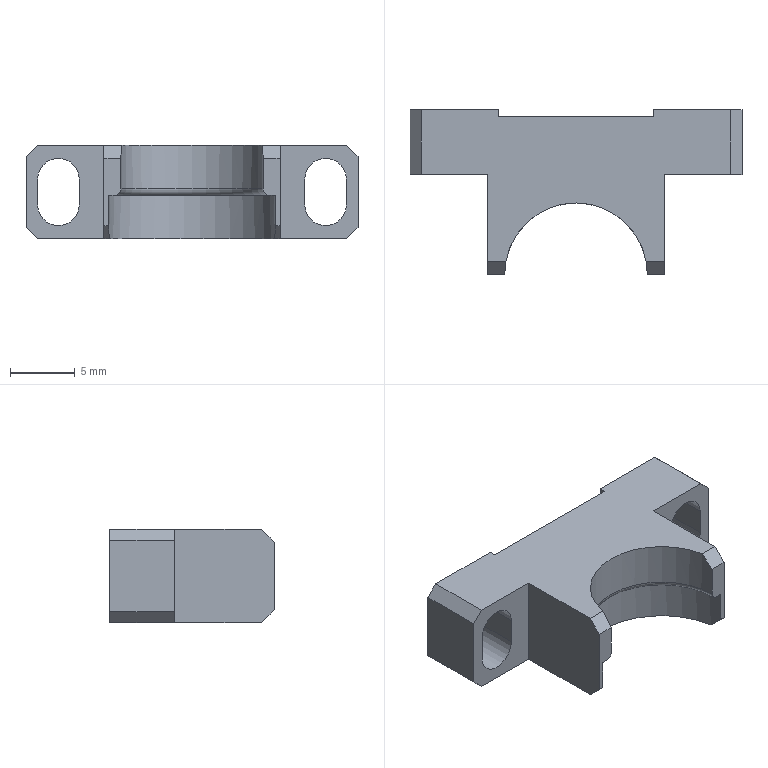Part | SolidWorks | features ICE 7, Chamfer 2, MoveFace 2, Extrusion 1, Fillet 1 | 1 solid | 35 faces | box 25.6 x 12.7 x 7.2 mm | volume 1076 mm3 | plane 28 | cylinder 6 | torus 1 | commonest cylinder face diameters 3.2 x4 11 x1 12.9 x1
STEP:
#1=CARTESIAN_POINT('',(12.8,12.7,5.995));
#2=VERTEX_POINT('',#1);
#3=CARTESIAN_POINT('',(12.8,12.7,0.505));
#4=VERTEX_POINT('',#3);
#5=CARTESIAN_POINT('',(12.8,12.7,0.));
#6=DIRECTION('',(0.,0.,-1.));
#7=VECTOR('',#6,1000.);
#8=LINE('',#5,#7);
#9=EDGE_CURVE('',#2,#4,#8,.T.);
#10=ORIENTED_EDGE('',*,*,#9,.T.);
#11=CARTESIAN_POINT('',(11.945,12.7,-0.35));
#12=VERTEX_POINT('',#11);
#13=CARTESIAN_POINT('',(9.547,12.7,-2.747));
#14=DIRECTION('',(-0.7071,0.,-0.7071));
#15=VECTOR('',#14,1000.);
#16=LINE('',#13,#15);
#17=EDGE_CURVE('',#4,#12,#16,.T.);
#18=ORIENTED_EDGE('',*,*,#17,.T.);
#19=CARTESIAN_POINT('',(6.,12.7,-0.35));
#20=VERTEX_POINT('',#19);
#21=CARTESIAN_POINT('',(0.,12.7,-0.35));
#22=DIRECTION('',(-1.,0.,0.));
#23=VECTOR('',#22,1000.);
#24=LINE('',#21,#23);
#25=EDGE_CURVE('',#12,#20,#24,.T.);
#26=ORIENTED_EDGE('',*,*,#25,.T.);
#27=CARTESIAN_POINT('',(6.,12.7,6.85));
#28=VERTEX_POINT('',#27);
#29=CARTESIAN_POINT('',(6.,12.7,0.));
#30=DIRECTION('',(0.,0.,-1.));
#31=VECTOR('',#30,1000.);
#32=LINE('',#29,#31);
#33=EDGE_CURVE('',#28,#20,#32,.T.);
#34=ORIENTED_EDGE('',*,*,#33,.F.);
#35=CARTESIAN_POINT('',(11.945,12.7,6.85));
#36=VERTEX_POINT('',#35);
#37=CARTESIAN_POINT('',(0.,12.7,6.85));
#38=DIRECTION('',(-1.,0.,0.));
#39=VECTOR('',#38,1000.);
#40=LINE('',#37,#39);
#41=EDGE_CURVE('',#36,#28,#40,.T.);
#42=ORIENTED_EDGE('',*,*,#41,.F.);
#43=CARTESIAN_POINT('',(12.797,12.7,5.997));
#44=DIRECTION('',(0.7071,0.,-0.7071));
#45=VECTOR('',#44,1000.);
#46=LINE('',#43,#45);
#47=EDGE_CURVE('',#36,#2,#46,.T.);
#48=ORIENTED_EDGE('',*,*,#47,.T.);
#49=EDGE_LOOP('',(#10,#18,#26,#34,#42,#48));
#50=FACE_OUTER_BOUND('',#49,.T.);
#51=CARTESIAN_POINT('',(8.7,12.7,2.25));
#52=VERTEX_POINT('',#51);
#53=CARTESIAN_POINT('',(11.9,12.7,2.25));
#54=VERTEX_POINT('',#53);
#55=CARTESIAN_POINT('',(10.3,12.7,2.25));
#56=DIRECTION('',(0.,-1.,0.));
#57=DIRECTION('',(1.,0.,0.));
#58=AXIS2_PLACEMENT_3D('',#55,#56,#57);
#59=CIRCLE('',#58,1.6);
#60=EDGE_CURVE('',#52,#54,#59,.T.);
#61=ORIENTED_EDGE('',*,*,#60,.T.);
#62=CARTESIAN_POINT('',(11.9,12.7,4.25));
#63=VERTEX_POINT('',#62);
#64=CARTESIAN_POINT('',(11.9,12.7,2.25));
#65=DIRECTION('',(0.,0.,1.));
#66=VECTOR('',#65,1000.);
#67=LINE('',#64,#66);
#68=EDGE_CURVE('',#54,#63,#67,.T.);
#69=ORIENTED_EDGE('',*,*,#68,.T.);
#70=CARTESIAN_POINT('',(8.7,12.7,4.25));
#71=VERTEX_POINT('',#70);
#72=CARTESIAN_POINT('',(10.3,12.7,4.25));
#73=DIRECTION('',(0.,-1.,0.));
#74=DIRECTION('',(1.,0.,0.));
#75=AXIS2_PLACEMENT_3D('',#72,#73,#74);
#76=CIRCLE('',#75,1.6);
#77=EDGE_CURVE('',#63,#71,#76,.T.);
#78=ORIENTED_EDGE('',*,*,#77,.T.);
#79=CARTESIAN_POINT('',(8.7,12.7,2.25));
#80=DIRECTION('',(0.,0.,-1.));
#81=VECTOR('',#80,1000.);
#82=LINE('',#79,#81);
#83=EDGE_CURVE('',#71,#52,#82,.T.);
#84=ORIENTED_EDGE('',*,*,#83,.T.);
#85=EDGE_LOOP('',(#61,#69,#78,#84));
#86=FACE_BOUND('',#85,.T.);
#87=CARTESIAN_POINT('',(6.8,12.7,0.));
#88=DIRECTION('',(0.,1.,0.));
#89=DIRECTION('',(-1.,0.,0.));
#90=AXIS2_PLACEMENT_3D('',#87,#88,#89);
#91=PLANE('',#90);
#92=ADVANCED_FACE('',(#50,#86),#91,.T.);
#93=CARTESIAN_POINT('',(-6.8,0.,0.65));
#94=VERTEX_POINT('',#93);
#95=CARTESIAN_POINT('',(-6.8,0.,5.85));
#96=VERTEX_POINT('',#95);
#97=CARTESIAN_POINT('',(-6.8,0.,0.));
#98=DIRECTION('',(0.,0.,1.));
#99=VECTOR('',#98,1000.);
#100=LINE('',#97,#99);
#101=EDGE_CURVE('',#94,#96,#100,.T.);
#102=ORIENTED_EDGE('',*,*,#101,.T.);
#103=CARTESIAN_POINT('',(-6.8,1.,6.85));
#104=VERTEX_POINT('',#103);
#105=CARTESIAN_POINT('',(-6.8,-2.925,2.925));
#106=DIRECTION('',(0.,0.7071,0.7071));
#107=VECTOR('',#106,1000.);
#108=LINE('',#105,#107);
#109=EDGE_CURVE('',#96,#104,#108,.T.);
#110=ORIENTED_EDGE('',*,*,#109,.T.);
#111=CARTESIAN_POINT('',(-6.8,7.7,6.85));
#112=VERTEX_POINT('',#111);
#113=CARTESIAN_POINT('',(-6.8,0.,6.85));
#114=DIRECTION('',(0.,-1.,0.));
#115=VECTOR('',#114,1000.);
#116=LINE('',#113,#115);
#117=EDGE_CURVE('',#112,#104,#116,.T.);
#118=ORIENTED_EDGE('',*,*,#117,.F.);
#119=CARTESIAN_POINT('',(-6.8,7.7,-0.35));
#120=VERTEX_POINT('',#119);
#121=CARTESIAN_POINT('',(-6.8,7.7,6.5));
#122=DIRECTION('',(0.,0.,-1.));
#123=VECTOR('',#122,1000.);
#124=LINE('',#121,#123);
#125=EDGE_CURVE('',#112,#120,#124,.T.);
#126=ORIENTED_EDGE('',*,*,#125,.T.);
#127=CARTESIAN_POINT('',(-6.8,1.,-0.35));
#128=VERTEX_POINT('',#127);
#129=CARTESIAN_POINT('',(-6.8,0.,-0.35));
#130=DIRECTION('',(0.,-1.,0.));
#131=VECTOR('',#130,1000.);
#132=LINE('',#129,#131);
#133=EDGE_CURVE('',#120,#128,#132,.T.);
#134=ORIENTED_EDGE('',*,*,#133,.T.);
#135=CARTESIAN_POINT('',(-6.8,0.325,0.325));
#136=DIRECTION('',(0.,-0.7071,0.7071));
#137=VECTOR('',#136,1000.);
#138=LINE('',#135,#137);
#139=EDGE_CURVE('',#128,#94,#138,.T.);
#140=ORIENTED_EDGE('',*,*,#139,.T.);
#141=EDGE_LOOP('',(#102,#110,#118,#126,#134,#140));
#142=FACE_OUTER_BOUND('',#141,.T.);
#143=CARTESIAN_POINT('',(-6.8,0.,0.));
#144=DIRECTION('',(-1.,0.,0.));
#145=DIRECTION('',(0.,0.,1.));
#146=AXIS2_PLACEMENT_3D('',#143,#144,#145);
#147=PLANE('',#146);
#148=ADVANCED_FACE('',(#142),#147,.T.);
#149=CARTESIAN_POINT('',(6.8,1.,6.85));
#150=VERTEX_POINT('',#149);
#151=CARTESIAN_POINT('',(6.8,7.7,6.85));
#152=VERTEX_POINT('',#151);
#153=CARTESIAN_POINT('',(6.8,0.,6.85));
#154=DIRECTION('',(0.,1.,0.));
#155=VECTOR('',#154,1000.);
#156=LINE('',#153,#155);
#157=EDGE_CURVE('',#150,#152,#156,.T.);
#158=ORIENTED_EDGE('',*,*,#157,.F.);
#159=CARTESIAN_POINT('',(6.8,0.,5.85));
#160=VERTEX_POINT('',#159);
#161=CARTESIAN_POINT('',(6.8,-2.925,2.925));
#162=DIRECTION('',(0.,-0.7071,-0.7071));
#163=VECTOR('',#162,1000.);
#164=LINE('',#161,#163);
#165=EDGE_CURVE('',#150,#160,#164,.T.);
#166=ORIENTED_EDGE('',*,*,#165,.T.);
#167=CARTESIAN_POINT('',(6.8,0.,0.65));
#168=VERTEX_POINT('',#167);
#169=CARTESIAN_POINT('',(6.8,0.,0.));
#170=DIRECTION('',(0.,0.,1.));
#171=VECTOR('',#170,1000.);
#172=LINE('',#169,#171);
#173=EDGE_CURVE('',#168,#160,#172,.T.);
#174=ORIENTED_EDGE('',*,*,#173,.F.);
#175=CARTESIAN_POINT('',(6.8,1.,-0.35));
#176=VERTEX_POINT('',#175);
#177=CARTESIAN_POINT('',(6.8,0.325,0.325));
#178=DIRECTION('',(0.,0.7071,-0.7071));
#179=VECTOR('',#178,1000.);
#180=LINE('',#177,#179);
#181=EDGE_CURVE('',#168,#176,#180,.T.);
#182=ORIENTED_EDGE('',*,*,#181,.T.);
#183=CARTESIAN_POINT('',(6.8,7.7,-0.35));
#184=VERTEX_POINT('',#183);
#185=CARTESIAN_POINT('',(6.8,0.,-0.35));
#186=DIRECTION('',(0.,1.,0.));
#187=VECTOR('',#186,1000.);
#188=LINE('',#185,#187);
#189=EDGE_CURVE('',#176,#184,#188,.T.);
#190=ORIENTED_EDGE('',*,*,#189,.T.);
#191=CARTESIAN_POINT('',(6.8,7.7,0.));
#192=DIRECTION('',(0.,0.,1.));
#193=VECTOR('',#192,1000.);
#194=LINE('',#191,#193);
#195=EDGE_CURVE('',#184,#152,#194,.T.);
#196=ORIENTED_EDGE('',*,*,#195,.T.);
#197=EDGE_LOOP('',(#158,#166,#174,#182,#190,#196));
#198=FACE_OUTER_BOUND('',#197,.T.);
#199=CARTESIAN_POINT('',(6.8,0.,0.));
#200=DIRECTION('',(1.,0.,0.));
#201=DIRECTION('',(0.,0.,-1.));
#202=AXIS2_PLACEMENT_3D('',#199,#200,#201);
#203=PLANE('',#202);
#204=ADVANCED_FACE('',(#198),#203,.T.);
#205=CARTESIAN_POINT('',(5.5,0.,3.5));
#206=VERTEX_POINT('',#205);
#207=CARTESIAN_POINT('',(5.5,0.,5.85));
#208=VERTEX_POINT('',#207);
#209=CARTESIAN_POINT('',(5.5,0.,10.));
#210=DIRECTION('',(0.,0.,1.));
#211=VECTOR('',#210,1000.);
#212=LINE('',#209,#211);
#213=EDGE_CURVE('',#206,#208,#212,.T.);
#214=ORIENTED_EDGE('',*,*,#213,.T.);
#215=CARTESIAN_POINT('',(5.408,1.,6.85));
#216=VERTEX_POINT('',#215);
#217=CARTESIAN_POINT('',(5.5,0.,5.85));
#218=CARTESIAN_POINT('',(5.5,0.3357,6.186));
#219=CARTESIAN_POINT('',(5.469,0.6699,6.52));
#220=CARTESIAN_POINT('',(5.408,1.,6.85));
#221=(BOUNDED_CURVE()B_SPLINE_CURVE(3,(#217,#218,#219,#220),.UNSPECIFIED.,.F.,.T.)B_SPLINE_CURVE_WITH_KNOTS((4,4),(1.571,1.754),.UNSPECIFIED.)CURVE()GEOMETRIC_REPRESENTATION_ITEM()RATIONAL_B_SPLINE_CURVE((1.,0.9972,0.9972,1.))REPRESENTATION_ITEM(''));
#222=EDGE_CURVE('',#208,#216,#221,.T.);
#223=ORIENTED_EDGE('',*,*,#222,.T.);
#224=CARTESIAN_POINT('',(-5.408,1.,6.85));
#225=VERTEX_POINT('',#224);
#226=CARTESIAN_POINT('',(0.,0.,6.85));
#227=DIRECTION('',(0.,0.,1.));
#228=DIRECTION('',(1.,0.,0.));
#229=AXIS2_PLACEMENT_3D('',#226,#227,#228);
#230=CIRCLE('',#229,5.5);
#231=EDGE_CURVE('',#216,#225,#230,.T.);
#232=ORIENTED_EDGE('',*,*,#231,.T.);
#233=CARTESIAN_POINT('',(-5.5,0.,5.85));
#234=VERTEX_POINT('',#233);
#235=CARTESIAN_POINT('',(-5.408,1.,6.85));
#236=CARTESIAN_POINT('',(-5.469,0.6699,6.52));
#237=CARTESIAN_POINT('',(-5.5,0.3357,6.186));
#238=CARTESIAN_POINT('',(-5.5,0.,5.85));
#239=(BOUNDED_CURVE()B_SPLINE_CURVE(3,(#235,#236,#237,#238),.UNSPECIFIED.,.F.,.F.)B_SPLINE_CURVE_WITH_KNOTS((4,4),(4.53,4.712),.UNSPECIFIED.)CURVE()GEOMETRIC_REPRESENTATION_ITEM()RATIONAL_B_SPLINE_CURVE((1.,0.9972,0.9972,1.))REPRESENTATION_ITEM(''));
#240=EDGE_CURVE('',#225,#234,#239,.T.);
#241=ORIENTED_EDGE('',*,*,#240,.T.);
#242=CARTESIAN_POINT('',(-5.5,0.,3.5));
#243=VERTEX_POINT('',#242);
#244=CARTESIAN_POINT('',(-5.5,0.,10.));
#245=DIRECTION('',(0.,0.,-1.));
#246=VECTOR('',#245,1000.);
#247=LINE('',#244,#246);
#248=EDGE_CURVE('',#234,#243,#247,.T.);
#249=ORIENTED_EDGE('',*,*,#248,.T.);
#250=CARTESIAN_POINT('',(0.,0.,3.5));
#251=DIRECTION('',(0.,0.,-1.));
#252=DIRECTION('',(-1.,0.,0.));
#253=AXIS2_PLACEMENT_3D('',#250,#251,#252);
#254=CIRCLE('',#253,5.5);
#255=EDGE_CURVE('',#243,#206,#254,.T.);
#256=ORIENTED_EDGE('',*,*,#255,.T.);
#257=EDGE_LOOP('',(#214,#223,#232,#241,#249,#256));
#258=FACE_OUTER_BOUND('',#257,.T.);
#259=CARTESIAN_POINT('',(0.,0.,10.));
#260=DIRECTION('',(0.,0.,-1.));
#261=DIRECTION('',(-1.,0.,0.));
#262=AXIS2_PLACEMENT_3D('',#259,#260,#261);
#263=CYLINDRICAL_SURFACE('',#262,5.5);
#264=ADVANCED_FACE('',(#258),#263,.F.);
#265=ORIENTED_EDGE('',*,*,#231,.F.);
#266=CARTESIAN_POINT('',(6.8,1.,6.85));
#267=DIRECTION('',(1.,0.,0.));
#268=VECTOR('',#267,1000.);
#269=LINE('',#266,#268);
#270=EDGE_CURVE('',#216,#150,#269,.T.);
#271=ORIENTED_EDGE('',*,*,#270,.T.);
#272=ORIENTED_EDGE('',*,*,#157,.T.);
#273=CARTESIAN_POINT('',(11.945,7.7,6.85));
#274=VERTEX_POINT('',#273);
#275=CARTESIAN_POINT('',(0.,7.7,6.85));
#276=DIRECTION('',(1.,0.,0.));
#277=VECTOR('',#276,1000.);
#278=LINE('',#275,#277);
#279=EDGE_CURVE('',#152,#274,#278,.T.);
#280=ORIENTED_EDGE('',*,*,#279,.T.);
#281=CARTESIAN_POINT('',(11.945,0.,6.85));
#282=DIRECTION('',(0.,1.,0.));
#283=VECTOR('',#282,1000.);
#284=LINE('',#281,#283);
#285=EDGE_CURVE('',#274,#36,#284,.T.);
#286=ORIENTED_EDGE('',*,*,#285,.T.);
#287=ORIENTED_EDGE('',*,*,#41,.T.);
#288=CARTESIAN_POINT('',(6.,12.2,6.85));
#289=VERTEX_POINT('',#288);
#290=CARTESIAN_POINT('',(6.,0.,6.85));
#291=DIRECTION('',(0.,1.,0.));
#292=VECTOR('',#291,1000.);
#293=LINE('',#290,#292);
#294=EDGE_CURVE('',#289,#28,#293,.T.);
#295=ORIENTED_EDGE('',*,*,#294,.F.);
#296=CARTESIAN_POINT('',(-6.,12.2,6.85));
#297=VERTEX_POINT('',#296);
#298=CARTESIAN_POINT('',(0.,12.2,6.85));
#299=DIRECTION('',(1.,0.,0.));
#300=VECTOR('',#299,1000.);
#301=LINE('',#298,#300);
#302=EDGE_CURVE('',#297,#289,#301,.T.);
#303=ORIENTED_EDGE('',*,*,#302,.F.);
#304=CARTESIAN_POINT('',(-6.,12.7,6.85));
#305=VERTEX_POINT('',#304);
#306=CARTESIAN_POINT('',(-6.,12.2,6.85));
#307=DIRECTION('',(0.,1.,0.));
#308=VECTOR('',#307,1000.);
#309=LINE('',#306,#308);
#310=EDGE_CURVE('',#297,#305,#309,.T.);
#311=ORIENTED_EDGE('',*,*,#310,.T.);
#312=CARTESIAN_POINT('',(-11.945,12.7,6.85));
#313=VERTEX_POINT('',#312);
#314=CARTESIAN_POINT('',(0.,12.7,6.85));
#315=DIRECTION('',(-1.,0.,0.));
#316=VECTOR('',#315,1000.);
#317=LINE('',#314,#316);
#318=EDGE_CURVE('',#305,#313,#317,.T.);
#319=ORIENTED_EDGE('',*,*,#318,.T.);
#320=CARTESIAN_POINT('',(-11.945,7.7,6.85));
#321=VERTEX_POINT('',#320);
#322=CARTESIAN_POINT('',(-11.945,0.,6.85));
#323=DIRECTION('',(0.,-1.,0.));
#324=VECTOR('',#323,1000.);
#325=LINE('',#322,#324);
#326=EDGE_CURVE('',#313,#321,#325,.T.);
#327=ORIENTED_EDGE('',*,*,#326,.T.);
#328=CARTESIAN_POINT('',(0.,7.7,6.85));
#329=DIRECTION('',(1.,0.,0.));
#330=VECTOR('',#329,1000.);
#331=LINE('',#328,#330);
#332=EDGE_CURVE('',#321,#112,#331,.T.);
#333=ORIENTED_EDGE('',*,*,#332,.T.);
#334=ORIENTED_EDGE('',*,*,#117,.T.);
#335=CARTESIAN_POINT('',(-5.5,1.,6.85));
#336=DIRECTION('',(1.,0.,0.));
#337=VECTOR('',#336,1000.);
#338=LINE('',#335,#337);
#339=EDGE_CURVE('',#104,#225,#338,.T.);
#340=ORIENTED_EDGE('',*,*,#339,.T.);
#341=EDGE_LOOP('',(#265,#271,#272,#280,#286,#287,#295,#303,#311,#319,#327,#333,#334,#340));
#342=FACE_OUTER_BOUND('',#341,.T.);
#343=CARTESIAN_POINT('',(0.,0.,6.85));
#344=DIRECTION('',(0.,0.,1.));
#345=DIRECTION('',(1.,0.,0.));
#346=AXIS2_PLACEMENT_3D('',#343,#344,#345);
#347=PLANE('',#346);
#348=ADVANCED_FACE('',(#342),#347,.T.);
#349=CARTESIAN_POINT('',(-6.372,1.,-0.35));
#350=VERTEX_POINT('',#349);
#351=CARTESIAN_POINT('',(6.372,1.,-0.35));
#352=VERTEX_POINT('',#351);
#353=CARTESIAN_POINT('',(0.,0.,-0.35));
#354=DIRECTION('',(0.,0.,-1.));
#355=DIRECTION('',(1.,0.,0.));
#356=AXIS2_PLACEMENT_3D('',#353,#354,#355);
#357=CIRCLE('',#356,6.45);
#358=EDGE_CURVE('',#350,#352,#357,.T.);
#359=ORIENTED_EDGE('',*,*,#358,.F.);
#360=CARTESIAN_POINT('',(0.,1.,-0.35));
#361=DIRECTION('',(-1.,0.,0.));
#362=VECTOR('',#361,1000.);
#363=LINE('',#360,#362);
#364=EDGE_CURVE('',#350,#128,#363,.T.);
#365=ORIENTED_EDGE('',*,*,#364,.T.);
#366=ORIENTED_EDGE('',*,*,#133,.F.);
#367=CARTESIAN_POINT('',(-11.945,7.7,-0.35));
#368=VERTEX_POINT('',#367);
#369=CARTESIAN_POINT('',(0.,7.7,-0.35));
#370=DIRECTION('',(-1.,0.,0.));
#371=VECTOR('',#370,1000.);
#372=LINE('',#369,#371);
#373=EDGE_CURVE('',#120,#368,#372,.T.);
#374=ORIENTED_EDGE('',*,*,#373,.T.);
#375=CARTESIAN_POINT('',(-11.945,12.7,-0.35));
#376=VERTEX_POINT('',#375);
#377=CARTESIAN_POINT('',(-11.945,0.,-0.35));
#378=DIRECTION('',(0.,1.,0.));
#379=VECTOR('',#378,1000.);
#380=LINE('',#377,#379);
#381=EDGE_CURVE('',#368,#376,#380,.T.);
#382=ORIENTED_EDGE('',*,*,#381,.T.);
#383=CARTESIAN_POINT('',(-6.,12.7,-0.35));
#384=VERTEX_POINT('',#383);
#385=CARTESIAN_POINT('',(0.,12.7,-0.35));
#386=DIRECTION('',(-1.,0.,0.));
#387=VECTOR('',#386,1000.);
#388=LINE('',#385,#387);
#389=EDGE_CURVE('',#384,#376,#388,.T.);
#390=ORIENTED_EDGE('',*,*,#389,.F.);
#391=CARTESIAN_POINT('',(-6.,12.2,-0.35));
#392=VERTEX_POINT('',#391);
#393=CARTESIAN_POINT('',(-6.,12.2,-0.35));
#394=DIRECTION('',(0.,1.,0.));
#395=VECTOR('',#394,1000.);
#396=LINE('',#393,#395);
#397=EDGE_CURVE('',#392,#384,#396,.T.);
#398=ORIENTED_EDGE('',*,*,#397,.F.);
#399=CARTESIAN_POINT('',(6.,12.2,-0.35));
#400=VERTEX_POINT('',#399);
#401=CARTESIAN_POINT('',(0.,12.2,-0.35));
#402=DIRECTION('',(-1.,0.,0.));
#403=VECTOR('',#402,1000.);
#404=LINE('',#401,#403);
#405=EDGE_CURVE('',#400,#392,#404,.T.);
#406=ORIENTED_EDGE('',*,*,#405,.F.);
#407=CARTESIAN_POINT('',(6.,0.,-0.35));
#408=DIRECTION('',(0.,1.,0.));
#409=VECTOR('',#408,1000.);
#410=LINE('',#407,#409);
#411=EDGE_CURVE('',#400,#20,#410,.T.);
#412=ORIENTED_EDGE('',*,*,#411,.T.);
#413=ORIENTED_EDGE('',*,*,#25,.F.);
#414=CARTESIAN_POINT('',(11.945,7.7,-0.35));
#415=VERTEX_POINT('',#414);
#416=CARTESIAN_POINT('',(11.945,7.7,-0.35));
#417=DIRECTION('',(0.,-1.,0.));
#418=VECTOR('',#417,1000.);
#419=LINE('',#416,#418);
#420=EDGE_CURVE('',#12,#415,#419,.T.);
#421=ORIENTED_EDGE('',*,*,#420,.T.);
#422=CARTESIAN_POINT('',(0.,7.7,-0.35));
#423=DIRECTION('',(-1.,0.,0.));
#424=VECTOR('',#423,1000.);
#425=LINE('',#422,#424);
#426=EDGE_CURVE('',#415,#184,#425,.T.);
#427=ORIENTED_EDGE('',*,*,#426,.T.);
#428=ORIENTED_EDGE('',*,*,#189,.F.);
#429=CARTESIAN_POINT('',(0.,1.,-0.35));
#430=DIRECTION('',(-1.,0.,0.));
#431=VECTOR('',#430,1000.);
#432=LINE('',#429,#431);
#433=EDGE_CURVE('',#176,#352,#432,.T.);
#434=ORIENTED_EDGE('',*,*,#433,.T.);
#435=EDGE_LOOP('',(#359,#365,#366,#374,#382,#390,#398,#406,#412,#413,#421,#427,#428,#434));
#436=FACE_OUTER_BOUND('',#435,.T.);
#437=CARTESIAN_POINT('',(0.,0.,-0.35));
#438=DIRECTION('',(0.,0.,1.));
#439=DIRECTION('',(1.,0.,0.));
#440=AXIS2_PLACEMENT_3D('',#437,#438,#439);
#441=PLANE('',#440);
#442=ADVANCED_FACE('',(#436),#441,.F.);
#443=CARTESIAN_POINT('',(6.,0.,3.));
#444=VERTEX_POINT('',#443);
#445=CARTESIAN_POINT('',(6.45,0.,3.));
#446=VERTEX_POINT('',#445);
#447=CARTESIAN_POINT('',(0.,0.,3.));
#448=DIRECTION('',(1.,0.,0.));
#449=VECTOR('',#448,1000.);
#450=LINE('',#447,#449);
#451=EDGE_CURVE('',#444,#446,#450,.T.);
#452=ORIENTED_EDGE('',*,*,#451,.F.);
#453=CARTESIAN_POINT('',(-6.,0.,3.));
#454=VERTEX_POINT('',#453);
#455=CARTESIAN_POINT('',(0.,0.,3.));
#456=DIRECTION('',(0.,0.,1.));
#457=DIRECTION('',(-1.,0.,0.));
#458=AXIS2_PLACEMENT_3D('',#455,#456,#457);
#459=CIRCLE('',#458,6.);
#460=EDGE_CURVE('',#444,#454,#459,.T.);
#461=ORIENTED_EDGE('',*,*,#460,.T.);
#462=CARTESIAN_POINT('',(-6.45,0.,3.));
#463=VERTEX_POINT('',#462);
#464=CARTESIAN_POINT('',(0.,0.,3.));
#465=DIRECTION('',(1.,0.,0.));
#466=VECTOR('',#465,1000.);
#467=LINE('',#464,#466);
#468=EDGE_CURVE('',#463,#454,#467,.T.);
#469=ORIENTED_EDGE('',*,*,#468,.F.);
#470=CARTESIAN_POINT('',(0.,0.,3.));
#471=DIRECTION('',(0.,0.,-1.));
#472=DIRECTION('',(-1.,0.,0.));
#473=AXIS2_PLACEMENT_3D('',#470,#471,#472);
#474=CIRCLE('',#473,6.45);
#475=EDGE_CURVE('',#463,#446,#474,.T.);
#476=ORIENTED_EDGE('',*,*,#475,.T.);
#477=EDGE_LOOP('',(#452,#461,#469,#476));
#478=FACE_OUTER_BOUND('',#477,.T.);
#479=CARTESIAN_POINT('',(0.,0.,3.));
#480=DIRECTION('',(0.,0.,-1.));
#481=DIRECTION('',(-1.,0.,0.));
#482=AXIS2_PLACEMENT_3D('',#479,#480,#481);
#483=PLANE('',#482);
#484=ADVANCED_FACE('',(#478),#483,.T.);
#485=CARTESIAN_POINT('',(-6.45,0.,0.65));
#486=VERTEX_POINT('',#485);
#487=CARTESIAN_POINT('',(-6.45,0.,3.));
#488=DIRECTION('',(0.,0.,-1.));
#489=VECTOR('',#488,1000.);
#490=LINE('',#487,#489);
#491=EDGE_CURVE('',#463,#486,#490,.T.);
#492=ORIENTED_EDGE('',*,*,#491,.T.);
#493=CARTESIAN_POINT('',(-6.45,0.,0.65));
#494=CARTESIAN_POINT('',(-6.45,0.335,0.315));
#495=CARTESIAN_POINT('',(-6.424,0.669,-0.01903));
#496=CARTESIAN_POINT('',(-6.372,1.,-0.35));
#497=(BOUNDED_CURVE()B_SPLINE_CURVE(3,(#493,#494,#495,#496),.UNSPECIFIED.,.F.,.F.)B_SPLINE_CURVE_WITH_KNOTS((4,4),(4.712,4.868),.UNSPECIFIED.)CURVE()GEOMETRIC_REPRESENTATION_ITEM()RATIONAL_B_SPLINE_CURVE((1.,0.998,0.998,1.))REPRESENTATION_ITEM(''));
#498=EDGE_CURVE('',#486,#350,#497,.T.);
#499=ORIENTED_EDGE('',*,*,#498,.T.);
#500=ORIENTED_EDGE('',*,*,#358,.T.);
#501=CARTESIAN_POINT('',(6.45,0.,0.65));
#502=VERTEX_POINT('',#501);
#503=CARTESIAN_POINT('',(6.372,1.,-0.35));
#504=CARTESIAN_POINT('',(6.424,0.669,-0.01903));
#505=CARTESIAN_POINT('',(6.45,0.335,0.315));
#506=CARTESIAN_POINT('',(6.45,0.,0.65));
#507=(BOUNDED_CURVE()B_SPLINE_CURVE(3,(#503,#504,#505,#506),.UNSPECIFIED.,.F.,.F.)B_SPLINE_CURVE_WITH_KNOTS((4,4),(1.415,1.571),.UNSPECIFIED.)CURVE()GEOMETRIC_REPRESENTATION_ITEM()RATIONAL_B_SPLINE_CURVE((1.,0.998,0.998,1.))REPRESENTATION_ITEM(''));
#508=EDGE_CURVE('',#352,#502,#507,.T.);
#509=ORIENTED_EDGE('',*,*,#508,.T.);
#510=CARTESIAN_POINT('',(6.45,0.,3.));
#511=DIRECTION('',(0.,0.,1.));
#512=VECTOR('',#511,1000.);
#513=LINE('',#510,#512);
#514=EDGE_CURVE('',#502,#446,#513,.T.);
#515=ORIENTED_EDGE('',*,*,#514,.T.);
#516=ORIENTED_EDGE('',*,*,#475,.F.);
#517=EDGE_LOOP('',(#492,#499,#500,#509,#515,#516));
#518=FACE_OUTER_BOUND('',#517,.T.);
#519=CARTESIAN_POINT('',(0.,0.,3.));
#520=DIRECTION('',(0.,0.,-1.));
#521=DIRECTION('',(-1.,0.,0.));
#522=AXIS2_PLACEMENT_3D('',#519,#520,#521);
#523=CYLINDRICAL_SURFACE('',#522,6.45);
#524=ADVANCED_FACE('',(#518),#523,.F.);
#525=CARTESIAN_POINT('',(-12.8,12.7,0.505));
#526=VERTEX_POINT('',#525);
#527=CARTESIAN_POINT('',(-12.8,12.7,5.995));
#528=VERTEX_POINT('',#527);
#529=CARTESIAN_POINT('',(-12.8,12.7,6.5));
#530=DIRECTION('',(0.,0.,1.));
#531=VECTOR('',#530,1000.);
#532=LINE('',#529,#531);
#533=EDGE_CURVE('',#526,#528,#532,.T.);
#534=ORIENTED_EDGE('',*,*,#533,.T.);
#535=CARTESIAN_POINT('',(-5.997,12.7,12.797));
#536=DIRECTION('',(0.7071,0.,0.7071));
#537=VECTOR('',#536,1000.);
#538=LINE('',#535,#537);
#539=EDGE_CURVE('',#528,#313,#538,.T.);
#540=ORIENTED_EDGE('',*,*,#539,.T.);
#541=ORIENTED_EDGE('',*,*,#318,.F.);
#542=CARTESIAN_POINT('',(-6.,12.7,6.5));
#543=DIRECTION('',(0.,0.,1.));
#544=VECTOR('',#543,1000.);
#545=LINE('',#542,#544);
#546=EDGE_CURVE('',#384,#305,#545,.T.);
#547=ORIENTED_EDGE('',*,*,#546,.F.);
#548=ORIENTED_EDGE('',*,*,#389,.T.);
#549=CARTESIAN_POINT('',(-2.747,12.7,-9.547));
#550=DIRECTION('',(-0.7071,0.,0.7071));
#551=VECTOR('',#550,1000.);
#552=LINE('',#549,#551);
#553=EDGE_CURVE('',#376,#526,#552,.T.);
#554=ORIENTED_EDGE('',*,*,#553,.T.);
#555=EDGE_LOOP('',(#534,#540,#541,#547,#548,#554));
#556=FACE_OUTER_BOUND('',#555,.T.);
#557=CARTESIAN_POINT('',(-8.7,12.7,4.25));
#558=VERTEX_POINT('',#557);
#559=CARTESIAN_POINT('',(-11.9,12.7,4.25));
#560=VERTEX_POINT('',#559);
#561=CARTESIAN_POINT('',(-10.3,12.7,4.25));
#562=DIRECTION('',(0.,-1.,0.));
#563=DIRECTION('',(-1.,0.,0.));
#564=AXIS2_PLACEMENT_3D('',#561,#562,#563);
#565=CIRCLE('',#564,1.6);
#566=EDGE_CURVE('',#558,#560,#565,.T.);
#567=ORIENTED_EDGE('',*,*,#566,.T.);
#568=CARTESIAN_POINT('',(-11.9,12.7,2.25));
#569=VERTEX_POINT('',#568);
#570=CARTESIAN_POINT('',(-11.9,12.7,2.25));
#571=DIRECTION('',(0.,0.,-1.));
#572=VECTOR('',#571,1000.);
#573=LINE('',#570,#572);
#574=EDGE_CURVE('',#560,#569,#573,.T.);
#575=ORIENTED_EDGE('',*,*,#574,.T.);
#576=CARTESIAN_POINT('',(-8.7,12.7,2.25));
#577=VERTEX_POINT('',#576);
#578=CARTESIAN_POINT('',(-10.3,12.7,2.25));
#579=DIRECTION('',(0.,-1.,0.));
#580=DIRECTION('',(-1.,0.,0.));
#581=AXIS2_PLACEMENT_3D('',#578,#579,#580);
#582=CIRCLE('',#581,1.6);
#583=EDGE_CURVE('',#569,#577,#582,.T.);
#584=ORIENTED_EDGE('',*,*,#583,.T.);
#585=CARTESIAN_POINT('',(-8.7,12.7,2.25));
#586=DIRECTION('',(0.,0.,1.));
#587=VECTOR('',#586,1000.);
#588=LINE('',#585,#587);
#589=EDGE_CURVE('',#577,#558,#588,.T.);
#590=ORIENTED_EDGE('',*,*,#589,.T.);
#591=EDGE_LOOP('',(#567,#575,#584,#590));
#592=FACE_BOUND('',#591,.T.);
#593=CARTESIAN_POINT('',(6.8,12.7,0.));
#594=DIRECTION('',(0.,1.,0.));
#595=DIRECTION('',(-1.,0.,0.));
#596=AXIS2_PLACEMENT_3D('',#593,#594,#595);
#597=PLANE('',#596);
#598=ADVANCED_FACE('',(#556,#592),#597,.T.);
#599=CARTESIAN_POINT('',(12.8,7.7,5.995));
#600=VERTEX_POINT('',#599);
#601=CARTESIAN_POINT('',(12.8,7.7,0.505));
#602=VERTEX_POINT('',#601);
#603=CARTESIAN_POINT('',(12.8,7.7,0.));
#604=DIRECTION('',(0.,0.,-1.));
#605=VECTOR('',#604,1000.);
#606=LINE('',#603,#605);
#607=EDGE_CURVE('',#600,#602,#606,.T.);
#608=ORIENTED_EDGE('',*,*,#607,.T.);
#609=CARTESIAN_POINT('',(12.8,7.7,0.505));
#610=DIRECTION('',(0.,1.,0.));
#611=VECTOR('',#610,1000.);
#612=LINE('',#609,#611);
#613=EDGE_CURVE('',#602,#4,#612,.T.);
#614=ORIENTED_EDGE('',*,*,#613,.T.);
#615=ORIENTED_EDGE('',*,*,#9,.F.);
#616=CARTESIAN_POINT('',(12.8,7.7,5.995));
#617=DIRECTION('',(0.,-1.,0.));
#618=VECTOR('',#617,1000.);
#619=LINE('',#616,#618);
#620=EDGE_CURVE('',#2,#600,#619,.T.);
#621=ORIENTED_EDGE('',*,*,#620,.T.);
#622=EDGE_LOOP('',(#608,#614,#615,#621));
#623=FACE_OUTER_BOUND('',#622,.T.);
#624=CARTESIAN_POINT('',(12.8,7.7,0.));
#625=DIRECTION('',(1.,0.,0.));
#626=DIRECTION('',(0.,0.,-1.));
#627=AXIS2_PLACEMENT_3D('',#624,#625,#626);
#628=PLANE('',#627);
#629=ADVANCED_FACE('',(#623),#628,.T.);
#630=CARTESIAN_POINT('',(11.9,7.7,2.25));
#631=VERTEX_POINT('',#630);
#632=CARTESIAN_POINT('',(11.9,7.7,4.25));
#633=VERTEX_POINT('',#632);
#634=CARTESIAN_POINT('',(11.9,7.7,2.25));
#635=DIRECTION('',(0.,0.,1.));
#636=VECTOR('',#635,1000.);
#637=LINE('',#634,#636);
#638=EDGE_CURVE('',#631,#633,#637,.T.);
#639=ORIENTED_EDGE('',*,*,#638,.F.);
#640=CARTESIAN_POINT('',(8.7,7.7,2.25));
#641=VERTEX_POINT('',#640);
#642=CARTESIAN_POINT('',(10.3,7.7,2.25));
#643=DIRECTION('',(0.,-1.,0.));
#644=DIRECTION('',(1.,0.,0.));
#645=AXIS2_PLACEMENT_3D('',#642,#643,#644);
#646=CIRCLE('',#645,1.6);
#647=EDGE_CURVE('',#641,#631,#646,.T.);
#648=ORIENTED_EDGE('',*,*,#647,.F.);
#649=CARTESIAN_POINT('',(8.7,7.7,4.25));
#650=VERTEX_POINT('',#649);
#651=CARTESIAN_POINT('',(8.7,7.7,2.25));
#652=DIRECTION('',(0.,0.,-1.));
#653=VECTOR('',#652,1000.);
#654=LINE('',#651,#653);
#655=EDGE_CURVE('',#650,#641,#654,.T.);
#656=ORIENTED_EDGE('',*,*,#655,.F.);
#657=CARTESIAN_POINT('',(10.3,7.7,4.25));
#658=DIRECTION('',(0.,-1.,0.));
#659=DIRECTION('',(1.,0.,0.));
#660=AXIS2_PLACEMENT_3D('',#657,#658,#659);
#661=CIRCLE('',#660,1.6);
#662=EDGE_CURVE('',#633,#650,#661,.T.);
#663=ORIENTED_EDGE('',*,*,#662,.F.);
#664=EDGE_LOOP('',(#639,#648,#656,#663));
#665=FACE_BOUND('',#664,.T.);
#666=ORIENTED_EDGE('',*,*,#426,.F.);
#667=CARTESIAN_POINT('',(13.047,7.7,0.7525));
#668=DIRECTION('',(0.7071,0.,0.7071));
#669=VECTOR('',#668,1000.);
#670=LINE('',#667,#669);
#671=EDGE_CURVE('',#415,#602,#670,.T.);
#672=ORIENTED_EDGE('',*,*,#671,.T.);
#673=ORIENTED_EDGE('',*,*,#607,.F.);
#674=CARTESIAN_POINT('',(12.047,7.7,6.747));
#675=DIRECTION('',(-0.7071,0.,0.7071));
#676=VECTOR('',#675,1000.);
#677=LINE('',#674,#676);
#678=EDGE_CURVE('',#600,#274,#677,.T.);
#679=ORIENTED_EDGE('',*,*,#678,.T.);
#680=ORIENTED_EDGE('',*,*,#279,.F.);
#681=ORIENTED_EDGE('',*,*,#195,.F.);
#682=EDGE_LOOP('',(#666,#672,#673,#679,#680,#681));
#683=FACE_OUTER_BOUND('',#682,.T.);
#684=CARTESIAN_POINT('',(0.,7.7,0.));
#685=DIRECTION('',(0.,1.,0.));
#686=DIRECTION('',(-1.,0.,0.));
#687=AXIS2_PLACEMENT_3D('',#684,#685,#686);
#688=PLANE('',#687);
#689=ADVANCED_FACE('',(#665,#683),#688,.F.);
#690=CARTESIAN_POINT('',(-12.8,7.7,0.505));
#691=VERTEX_POINT('',#690);
#692=CARTESIAN_POINT('',(-12.8,7.7,5.995));
#693=VERTEX_POINT('',#692);
#694=CARTESIAN_POINT('',(-12.8,7.7,6.5));
#695=DIRECTION('',(0.,0.,1.));
#696=VECTOR('',#695,1000.);
#697=LINE('',#694,#696);
#698=EDGE_CURVE('',#691,#693,#697,.T.);
#699=ORIENTED_EDGE('',*,*,#698,.T.);
#700=CARTESIAN_POINT('',(-12.8,7.7,5.995));
#701=DIRECTION('',(0.,1.,0.));
#702=VECTOR('',#701,1000.);
#703=LINE('',#700,#702);
#704=EDGE_CURVE('',#693,#528,#703,.T.);
#705=ORIENTED_EDGE('',*,*,#704,.T.);
#706=ORIENTED_EDGE('',*,*,#533,.F.);
#707=CARTESIAN_POINT('',(-12.8,7.7,0.505));
#708=DIRECTION('',(0.,-1.,0.));
#709=VECTOR('',#708,1000.);
#710=LINE('',#707,#709);
#711=EDGE_CURVE('',#526,#691,#710,.T.);
#712=ORIENTED_EDGE('',*,*,#711,.T.);
#713=EDGE_LOOP('',(#699,#705,#706,#712));
#714=FACE_OUTER_BOUND('',#713,.T.);
#715=CARTESIAN_POINT('',(-12.8,7.7,6.5));
#716=DIRECTION('',(-1.,0.,0.));
#717=DIRECTION('',(0.,-1.,0.));
#718=AXIS2_PLACEMENT_3D('',#715,#716,#717);
#719=PLANE('',#718);
#720=ADVANCED_FACE('',(#714),#719,.T.);
#721=CARTESIAN_POINT('',(-11.9,7.7,4.25));
#722=VERTEX_POINT('',#721);
#723=CARTESIAN_POINT('',(-11.9,7.7,2.25));
#724=VERTEX_POINT('',#723);
#725=CARTESIAN_POINT('',(-11.9,7.7,2.25));
#726=DIRECTION('',(0.,0.,-1.));
#727=VECTOR('',#726,1000.);
#728=LINE('',#725,#727);
#729=EDGE_CURVE('',#722,#724,#728,.T.);
#730=ORIENTED_EDGE('',*,*,#729,.F.);
#731=CARTESIAN_POINT('',(-8.7,7.7,4.25));
#732=VERTEX_POINT('',#731);
#733=CARTESIAN_POINT('',(-10.3,7.7,4.25));
#734=DIRECTION('',(0.,-1.,0.));
#735=DIRECTION('',(-1.,0.,0.));
#736=AXIS2_PLACEMENT_3D('',#733,#734,#735);
#737=CIRCLE('',#736,1.6);
#738=EDGE_CURVE('',#732,#722,#737,.T.);
#739=ORIENTED_EDGE('',*,*,#738,.F.);
#740=CARTESIAN_POINT('',(-8.7,7.7,2.25));
#741=VERTEX_POINT('',#740);
#742=CARTESIAN_POINT('',(-8.7,7.7,2.25));
#743=DIRECTION('',(0.,0.,1.));
#744=VECTOR('',#743,1000.);
#745=LINE('',#742,#744);
#746=EDGE_CURVE('',#741,#732,#745,.T.);
#747=ORIENTED_EDGE('',*,*,#746,.F.);
#748=CARTESIAN_POINT('',(-10.3,7.7,2.25));
#749=DIRECTION('',(0.,-1.,0.));
#750=DIRECTION('',(-1.,0.,0.));
#751=AXIS2_PLACEMENT_3D('',#748,#749,#750);
#752=CIRCLE('',#751,1.6);
#753=EDGE_CURVE('',#724,#741,#752,.T.);
#754=ORIENTED_EDGE('',*,*,#753,.F.);
#755=EDGE_LOOP('',(#730,#739,#747,#754));
#756=FACE_BOUND('',#755,.T.);
#757=ORIENTED_EDGE('',*,*,#332,.F.);
#758=CARTESIAN_POINT('',(-13.047,7.7,5.747));
#759=DIRECTION('',(-0.7071,0.,-0.7071));
#760=VECTOR('',#759,1000.);
#761=LINE('',#758,#760);
#762=EDGE_CURVE('',#321,#693,#761,.T.);
#763=ORIENTED_EDGE('',*,*,#762,.T.);
#764=ORIENTED_EDGE('',*,*,#698,.F.);
#765=CARTESIAN_POINT('',(-12.047,7.7,-0.2475));
#766=DIRECTION('',(0.7071,0.,-0.7071));
#767=VECTOR('',#766,1000.);
#768=LINE('',#765,#767);
#769=EDGE_CURVE('',#691,#368,#768,.T.);
#770=ORIENTED_EDGE('',*,*,#769,.T.);
#771=ORIENTED_EDGE('',*,*,#373,.F.);
#772=ORIENTED_EDGE('',*,*,#125,.F.);
#773=EDGE_LOOP('',(#757,#763,#764,#770,#771,#772));
#774=FACE_OUTER_BOUND('',#773,.T.);
#775=CARTESIAN_POINT('',(0.,7.7,0.));
#776=DIRECTION('',(0.,1.,0.));
#777=DIRECTION('',(-1.,0.,0.));
#778=AXIS2_PLACEMENT_3D('',#775,#776,#777);
#779=PLANE('',#778);
#780=ADVANCED_FACE('',(#756,#774),#779,.F.);
#781=ORIENTED_EDGE('',*,*,#738,.T.);
#782=CARTESIAN_POINT('',(-11.9,12.7,4.25));
#783=DIRECTION('',(0.,-1.,0.));
#784=VECTOR('',#783,1000.);
#785=LINE('',#782,#784);
#786=EDGE_CURVE('',#560,#722,#785,.T.);
#787=ORIENTED_EDGE('',*,*,#786,.F.);
#788=ORIENTED_EDGE('',*,*,#566,.F.);
#789=CARTESIAN_POINT('',(-8.7,12.7,4.25));
#790=DIRECTION('',(0.,-1.,0.));
#791=VECTOR('',#790,1000.);
#792=LINE('',#789,#791);
#793=EDGE_CURVE('',#558,#732,#792,.T.);
#794=ORIENTED_EDGE('',*,*,#793,.T.);
#795=EDGE_LOOP('',(#781,#787,#788,#794));
#796=FACE_OUTER_BOUND('',#795,.T.);
#797=CARTESIAN_POINT('',(-10.3,12.7,4.25));
#798=DIRECTION('',(0.,-1.,0.));
#799=DIRECTION('',(1.,0.,0.));
#800=AXIS2_PLACEMENT_3D('',#797,#798,#799);
#801=CYLINDRICAL_SURFACE('',#800,1.6);
#802=ADVANCED_FACE('',(#796),#801,.F.);
#803=ORIENTED_EDGE('',*,*,#746,.T.);
#804=ORIENTED_EDGE('',*,*,#793,.F.);
#805=ORIENTED_EDGE('',*,*,#589,.F.);
#806=CARTESIAN_POINT('',(-8.7,12.7,2.25));
#807=DIRECTION('',(0.,-1.,0.));
#808=VECTOR('',#807,1000.);
#809=LINE('',#806,#808);
#810=EDGE_CURVE('',#577,#741,#809,.T.);
#811=ORIENTED_EDGE('',*,*,#810,.T.);
#812=EDGE_LOOP('',(#803,#804,#805,#811));
#813=FACE_OUTER_BOUND('',#812,.T.);
#814=CARTESIAN_POINT('',(-8.7,12.7,2.25));
#815=DIRECTION('',(1.,0.,0.));
#816=DIRECTION('',(0.,1.,0.));
#817=AXIS2_PLACEMENT_3D('',#814,#815,#816);
#818=PLANE('',#817);
#819=ADVANCED_FACE('',(#813),#818,.F.);
#820=ORIENTED_EDGE('',*,*,#753,.T.);
#821=ORIENTED_EDGE('',*,*,#810,.F.);
#822=ORIENTED_EDGE('',*,*,#583,.F.);
#823=CARTESIAN_POINT('',(-11.9,12.7,2.25));
#824=DIRECTION('',(0.,-1.,0.));
#825=VECTOR('',#824,1000.);
#826=LINE('',#823,#825);
#827=EDGE_CURVE('',#569,#724,#826,.T.);
#828=ORIENTED_EDGE('',*,*,#827,.T.);
#829=EDGE_LOOP('',(#820,#821,#822,#828));
#830=FACE_OUTER_BOUND('',#829,.T.);
#831=CARTESIAN_POINT('',(-10.3,12.7,2.25));
#832=DIRECTION('',(0.,-1.,0.));
#833=DIRECTION('',(1.,0.,0.));
#834=AXIS2_PLACEMENT_3D('',#831,#832,#833);
#835=CYLINDRICAL_SURFACE('',#834,1.6);
#836=ADVANCED_FACE('',(#830),#835,.F.);
#837=ORIENTED_EDGE('',*,*,#729,.T.);
#838=ORIENTED_EDGE('',*,*,#827,.F.);
#839=ORIENTED_EDGE('',*,*,#574,.F.);
#840=ORIENTED_EDGE('',*,*,#786,.T.);
#841=EDGE_LOOP('',(#837,#838,#839,#840));
#842=FACE_OUTER_BOUND('',#841,.T.);
#843=CARTESIAN_POINT('',(-11.9,12.7,2.25));
#844=DIRECTION('',(-1.,0.,0.));
#845=DIRECTION('',(0.,-1.,0.));
#846=AXIS2_PLACEMENT_3D('',#843,#844,#845);
#847=PLANE('',#846);
#848=ADVANCED_FACE('',(#842),#847,.F.);
#849=ORIENTED_EDGE('',*,*,#647,.T.);
#850=CARTESIAN_POINT('',(11.9,12.7,2.25));
#851=DIRECTION('',(0.,-1.,0.));
#852=VECTOR('',#851,1000.);
#853=LINE('',#850,#852);
#854=EDGE_CURVE('',#54,#631,#853,.T.);
#855=ORIENTED_EDGE('',*,*,#854,.F.);
#856=ORIENTED_EDGE('',*,*,#60,.F.);
#857=CARTESIAN_POINT('',(8.7,12.7,2.25));
#858=DIRECTION('',(0.,-1.,0.));
#859=VECTOR('',#858,1000.);
#860=LINE('',#857,#859);
#861=EDGE_CURVE('',#52,#641,#860,.T.);
#862=ORIENTED_EDGE('',*,*,#861,.T.);
#863=EDGE_LOOP('',(#849,#855,#856,#862));
#864=FACE_OUTER_BOUND('',#863,.T.);
#865=CARTESIAN_POINT('',(10.3,12.7,2.25));
#866=DIRECTION('',(0.,-1.,0.));
#867=DIRECTION('',(1.,0.,0.));
#868=AXIS2_PLACEMENT_3D('',#865,#866,#867);
#869=CYLINDRICAL_SURFACE('',#868,1.6);
#870=ADVANCED_FACE('',(#864),#869,.F.);
#871=ORIENTED_EDGE('',*,*,#655,.T.);
#872=ORIENTED_EDGE('',*,*,#861,.F.);
#873=ORIENTED_EDGE('',*,*,#83,.F.);
#874=CARTESIAN_POINT('',(8.7,12.7,4.25));
#875=DIRECTION('',(0.,-1.,0.));
#876=VECTOR('',#875,1000.);
#877=LINE('',#874,#876);
#878=EDGE_CURVE('',#71,#650,#877,.T.);
#879=ORIENTED_EDGE('',*,*,#878,.T.);
#880=EDGE_LOOP('',(#871,#872,#873,#879));
#881=FACE_OUTER_BOUND('',#880,.T.);
#882=CARTESIAN_POINT('',(8.7,12.7,2.25));
#883=DIRECTION('',(-1.,0.,0.));
#884=DIRECTION('',(0.,-1.,0.));
#885=AXIS2_PLACEMENT_3D('',#882,#883,#884);
#886=PLANE('',#885);
#887=ADVANCED_FACE('',(#881),#886,.F.);
#888=ORIENTED_EDGE('',*,*,#662,.T.);
#889=ORIENTED_EDGE('',*,*,#878,.F.);
#890=ORIENTED_EDGE('',*,*,#77,.F.);
#891=CARTESIAN_POINT('',(11.9,12.7,4.25));
#892=DIRECTION('',(0.,-1.,0.));
#893=VECTOR('',#892,1000.);
#894=LINE('',#891,#893);
#895=EDGE_CURVE('',#63,#633,#894,.T.);
#896=ORIENTED_EDGE('',*,*,#895,.T.);
#897=EDGE_LOOP('',(#888,#889,#890,#896));
#898=FACE_OUTER_BOUND('',#897,.T.);
#899=CARTESIAN_POINT('',(10.3,12.7,4.25));
#900=DIRECTION('',(0.,-1.,0.));
#901=DIRECTION('',(1.,0.,0.));
#902=AXIS2_PLACEMENT_3D('',#899,#900,#901);
#903=CYLINDRICAL_SURFACE('',#902,1.6);
#904=ADVANCED_FACE('',(#898),#903,.F.);
#905=ORIENTED_EDGE('',*,*,#638,.T.);
#906=ORIENTED_EDGE('',*,*,#895,.F.);
#907=ORIENTED_EDGE('',*,*,#68,.F.);
#908=ORIENTED_EDGE('',*,*,#854,.T.);
#909=EDGE_LOOP('',(#905,#906,#907,#908));
#910=FACE_OUTER_BOUND('',#909,.T.);
#911=CARTESIAN_POINT('',(11.9,12.7,2.25));
#912=DIRECTION('',(1.,0.,0.));
#913=DIRECTION('',(0.,1.,0.));
#914=AXIS2_PLACEMENT_3D('',#911,#912,#913);
#915=PLANE('',#914);
#916=ADVANCED_FACE('',(#910),#915,.F.);
#917=ORIENTED_EDGE('',*,*,#248,.F.);
#918=CARTESIAN_POINT('',(-6.8,0.,5.85));
#919=DIRECTION('',(-1.,0.,0.));
#920=VECTOR('',#919,1000.);
#921=LINE('',#918,#920);
#922=EDGE_CURVE('',#234,#96,#921,.T.);
#923=ORIENTED_EDGE('',*,*,#922,.T.);
#924=ORIENTED_EDGE('',*,*,#101,.F.);
#925=CARTESIAN_POINT('',(-6.8,0.,0.65));
#926=DIRECTION('',(1.,0.,0.));
#927=VECTOR('',#926,1000.);
#928=LINE('',#925,#927);
#929=EDGE_CURVE('',#94,#486,#928,.T.);
#930=ORIENTED_EDGE('',*,*,#929,.T.);
#931=ORIENTED_EDGE('',*,*,#491,.F.);
#932=ORIENTED_EDGE('',*,*,#468,.T.);
#933=CARTESIAN_POINT('',(-6.,0.,3.5));
#934=DIRECTION('',(0.,-1.,0.));
#935=DIRECTION('',(-1.,0.,0.));
#936=AXIS2_PLACEMENT_3D('',#933,#934,#935);
#937=CIRCLE('',#936,0.5);
#938=EDGE_CURVE('',#454,#243,#937,.T.);
#939=ORIENTED_EDGE('',*,*,#938,.T.);
#940=EDGE_LOOP('',(#917,#923,#924,#930,#931,#932,#939));
#941=FACE_OUTER_BOUND('',#940,.T.);
#942=CARTESIAN_POINT('',(-6.8,0.,10.));
#943=DIRECTION('',(0.,1.,0.));
#944=DIRECTION('',(-1.,0.,0.));
#945=AXIS2_PLACEMENT_3D('',#942,#943,#944);
#946=PLANE('',#945);
#947=ADVANCED_FACE('',(#941),#946,.F.);
#948=ORIENTED_EDGE('',*,*,#173,.T.);
#949=CARTESIAN_POINT('',(5.5,0.,5.85));
#950=DIRECTION('',(-1.,0.,0.));
#951=VECTOR('',#950,1000.);
#952=LINE('',#949,#951);
#953=EDGE_CURVE('',#160,#208,#952,.T.);
#954=ORIENTED_EDGE('',*,*,#953,.T.);
#955=ORIENTED_EDGE('',*,*,#213,.F.);
#956=CARTESIAN_POINT('',(6.,0.,3.5));
#957=DIRECTION('',(0.,-1.,0.));
#958=DIRECTION('',(-1.,0.,0.));
#959=AXIS2_PLACEMENT_3D('',#956,#957,#958);
#960=CIRCLE('',#959,0.5);
#961=EDGE_CURVE('',#206,#444,#960,.T.);
#962=ORIENTED_EDGE('',*,*,#961,.T.);
#963=ORIENTED_EDGE('',*,*,#451,.T.);
#964=ORIENTED_EDGE('',*,*,#514,.F.);
#965=CARTESIAN_POINT('',(-6.8,0.,0.65));
#966=DIRECTION('',(1.,0.,0.));
#967=VECTOR('',#966,1000.);
#968=LINE('',#965,#967);
#969=EDGE_CURVE('',#502,#168,#968,.T.);
#970=ORIENTED_EDGE('',*,*,#969,.T.);
#971=EDGE_LOOP('',(#948,#954,#955,#962,#963,#964,#970));
#972=FACE_OUTER_BOUND('',#971,.T.);
#973=CARTESIAN_POINT('',(-6.8,0.,10.));
#974=DIRECTION('',(0.,1.,0.));
#975=DIRECTION('',(-1.,0.,0.));
#976=AXIS2_PLACEMENT_3D('',#973,#974,#975);
#977=PLANE('',#976);
#978=ADVANCED_FACE('',(#972),#977,.F.);
#979=ORIENTED_EDGE('',*,*,#33,.T.);
#980=ORIENTED_EDGE('',*,*,#411,.F.);
#981=CARTESIAN_POINT('',(6.,12.2,0.));
#982=DIRECTION('',(0.,0.,-1.));
#983=VECTOR('',#982,1000.);
#984=LINE('',#981,#983);
#985=EDGE_CURVE('',#289,#400,#984,.T.);
#986=ORIENTED_EDGE('',*,*,#985,.F.);
#987=ORIENTED_EDGE('',*,*,#294,.T.);
#988=EDGE_LOOP('',(#979,#980,#986,#987));
#989=FACE_OUTER_BOUND('',#988,.T.);
#990=CARTESIAN_POINT('',(6.,12.2,0.));
#991=DIRECTION('',(1.,0.,0.));
#992=DIRECTION('',(0.,1.,0.));
#993=AXIS2_PLACEMENT_3D('',#990,#991,#992);
#994=PLANE('',#993);
#995=ADVANCED_FACE('',(#989),#994,.F.);
#996=ORIENTED_EDGE('',*,*,#546,.T.);
#997=ORIENTED_EDGE('',*,*,#310,.F.);
#998=CARTESIAN_POINT('',(-6.,12.2,6.5));
#999=DIRECTION('',(0.,0.,1.));
#1000=VECTOR('',#999,1000.);
#1001=LINE('',#998,#1000);
#1002=EDGE_CURVE('',#392,#297,#1001,.T.);
#1003=ORIENTED_EDGE('',*,*,#1002,.F.);
#1004=ORIENTED_EDGE('',*,*,#397,.T.);
#1005=EDGE_LOOP('',(#996,#997,#1003,#1004));
#1006=FACE_OUTER_BOUND('',#1005,.T.);
#1007=CARTESIAN_POINT('',(-6.,12.2,6.5));
#1008=DIRECTION('',(-1.,0.,0.));
#1009=DIRECTION('',(0.,0.,1.));
#1010=AXIS2_PLACEMENT_3D('',#1007,#1008,#1009);
#1011=PLANE('',#1010);
#1012=ADVANCED_FACE('',(#1006),#1011,.F.);
#1013=ORIENTED_EDGE('',*,*,#405,.T.);
#1014=ORIENTED_EDGE('',*,*,#1002,.T.);
#1015=ORIENTED_EDGE('',*,*,#302,.T.);
#1016=ORIENTED_EDGE('',*,*,#985,.T.);
#1017=EDGE_LOOP('',(#1013,#1014,#1015,#1016));
#1018=FACE_OUTER_BOUND('',#1017,.T.);
#1019=CARTESIAN_POINT('',(0.,12.2,0.));
#1020=DIRECTION('',(0.,-1.,0.));
#1021=DIRECTION('',(1.,0.,0.));
#1022=AXIS2_PLACEMENT_3D('',#1019,#1020,#1021);
#1023=PLANE('',#1022);
#1024=ADVANCED_FACE('',(#1018),#1023,.F.);
#1025=ORIENTED_EDGE('',*,*,#671,.F.);
#1026=ORIENTED_EDGE('',*,*,#420,.F.);
#1027=ORIENTED_EDGE('',*,*,#17,.F.);
#1028=ORIENTED_EDGE('',*,*,#613,.F.);
#1029=EDGE_LOOP('',(#1025,#1026,#1027,#1028));
#1030=FACE_OUTER_BOUND('',#1029,.T.);
#1031=CARTESIAN_POINT('',(13.047,7.7,0.7525));
#1032=DIRECTION('',(0.7071,0.,-0.7071));
#1033=DIRECTION('',(0.,-1.,0.));
#1034=AXIS2_PLACEMENT_3D('',#1031,#1032,#1033);
#1035=PLANE('',#1034);
#1036=ADVANCED_FACE('',(#1030),#1035,.T.);
#1037=ORIENTED_EDGE('',*,*,#678,.F.);
#1038=ORIENTED_EDGE('',*,*,#620,.F.);
#1039=ORIENTED_EDGE('',*,*,#47,.F.);
#1040=ORIENTED_EDGE('',*,*,#285,.F.);
#1041=EDGE_LOOP('',(#1037,#1038,#1039,#1040));
#1042=FACE_OUTER_BOUND('',#1041,.T.);
#1043=CARTESIAN_POINT('',(12.047,0.,6.747));
#1044=DIRECTION('',(-0.7071,0.,-0.7071));
#1045=DIRECTION('',(0.,1.,0.));
#1046=AXIS2_PLACEMENT_3D('',#1043,#1044,#1045);
#1047=PLANE('',#1046);
#1048=ADVANCED_FACE('',(#1042),#1047,.F.);
#1049=ORIENTED_EDGE('',*,*,#762,.F.);
#1050=ORIENTED_EDGE('',*,*,#326,.F.);
#1051=ORIENTED_EDGE('',*,*,#539,.F.);
#1052=ORIENTED_EDGE('',*,*,#704,.F.);
#1053=EDGE_LOOP('',(#1049,#1050,#1051,#1052));
#1054=FACE_OUTER_BOUND('',#1053,.T.);
#1055=CARTESIAN_POINT('',(-13.047,7.7,5.747));
#1056=DIRECTION('',(0.7071,0.,-0.7071));
#1057=DIRECTION('',(0.,1.,0.));
#1058=AXIS2_PLACEMENT_3D('',#1055,#1056,#1057);
#1059=PLANE('',#1058);
#1060=ADVANCED_FACE('',(#1054),#1059,.F.);
#1061=ORIENTED_EDGE('',*,*,#769,.F.);
#1062=ORIENTED_EDGE('',*,*,#711,.F.);
#1063=ORIENTED_EDGE('',*,*,#553,.F.);
#1064=ORIENTED_EDGE('',*,*,#381,.F.);
#1065=EDGE_LOOP('',(#1061,#1062,#1063,#1064));
#1066=FACE_OUTER_BOUND('',#1065,.T.);
#1067=CARTESIAN_POINT('',(-12.047,0.,-0.2475));
#1068=DIRECTION('',(-0.7071,0.,-0.7071));
#1069=DIRECTION('',(0.,-1.,0.));
#1070=AXIS2_PLACEMENT_3D('',#1067,#1068,#1069);
#1071=PLANE('',#1070);
#1072=ADVANCED_FACE('',(#1066),#1071,.T.);
#1073=ORIENTED_EDGE('',*,*,#961,.F.);
#1074=ORIENTED_EDGE('',*,*,#255,.F.);
#1075=ORIENTED_EDGE('',*,*,#938,.F.);
#1076=ORIENTED_EDGE('',*,*,#460,.F.);
#1077=EDGE_LOOP('',(#1073,#1074,#1075,#1076));
#1078=FACE_OUTER_BOUND('',#1077,.T.);
#1079=CARTESIAN_POINT('',(0.,0.,3.5));
#1080=DIRECTION('',(0.,0.,-1.));
#1081=DIRECTION('',(-1.,0.,0.));
#1082=AXIS2_PLACEMENT_3D('',#1079,#1080,#1081);
#1083=TOROIDAL_SURFACE('',#1082,6.,0.5);
#1084=ADVANCED_FACE('',(#1078),#1083,.T.);
#1085=ORIENTED_EDGE('',*,*,#165,.F.);
#1086=ORIENTED_EDGE('',*,*,#270,.F.);
#1087=ORIENTED_EDGE('',*,*,#222,.F.);
#1088=ORIENTED_EDGE('',*,*,#953,.F.);
#1089=EDGE_LOOP('',(#1085,#1086,#1087,#1088));
#1090=FACE_OUTER_BOUND('',#1089,.T.);
#1091=CARTESIAN_POINT('',(-6.8,0.,5.85));
#1092=DIRECTION('',(0.,-0.7071,0.7071));
#1093=DIRECTION('',(1.,0.,0.));
#1094=AXIS2_PLACEMENT_3D('',#1091,#1092,#1093);
#1095=PLANE('',#1094);
#1096=ADVANCED_FACE('',(#1090),#1095,.T.);
#1097=ORIENTED_EDGE('',*,*,#240,.F.);
#1098=ORIENTED_EDGE('',*,*,#339,.F.);
#1099=ORIENTED_EDGE('',*,*,#109,.F.);
#1100=ORIENTED_EDGE('',*,*,#922,.F.);
#1101=EDGE_LOOP('',(#1097,#1098,#1099,#1100));
#1102=FACE_OUTER_BOUND('',#1101,.T.);
#1103=CARTESIAN_POINT('',(-6.8,0.,5.85));
#1104=DIRECTION('',(0.,-0.7071,0.7071));
#1105=DIRECTION('',(1.,0.,0.));
#1106=AXIS2_PLACEMENT_3D('',#1103,#1104,#1105);
#1107=PLANE('',#1106);
#1108=ADVANCED_FACE('',(#1102),#1107,.T.);
#1109=ORIENTED_EDGE('',*,*,#139,.F.);
#1110=ORIENTED_EDGE('',*,*,#364,.F.);
#1111=ORIENTED_EDGE('',*,*,#498,.F.);
#1112=ORIENTED_EDGE('',*,*,#929,.F.);
#1113=EDGE_LOOP('',(#1109,#1110,#1111,#1112));
#1114=FACE_OUTER_BOUND('',#1113,.T.);
#1115=CARTESIAN_POINT('',(-6.8,0.,0.65));
#1116=DIRECTION('',(0.,0.7071,0.7071));
#1117=DIRECTION('',(1.,0.,0.));
#1118=AXIS2_PLACEMENT_3D('',#1115,#1116,#1117);
#1119=PLANE('',#1118);
#1120=ADVANCED_FACE('',(#1114),#1119,.F.);
#1121=ORIENTED_EDGE('',*,*,#508,.F.);
#1122=ORIENTED_EDGE('',*,*,#433,.F.);
#1123=ORIENTED_EDGE('',*,*,#181,.F.);
#1124=ORIENTED_EDGE('',*,*,#969,.F.);
#1125=EDGE_LOOP('',(#1121,#1122,#1123,#1124));
#1126=FACE_OUTER_BOUND('',#1125,.T.);
#1127=CARTESIAN_POINT('',(-6.8,0.,0.65));
#1128=DIRECTION('',(0.,0.7071,0.7071));
#1129=DIRECTION('',(1.,0.,0.));
#1130=AXIS2_PLACEMENT_3D('',#1127,#1128,#1129);
#1131=PLANE('',#1130);
#1132=ADVANCED_FACE('',(#1126),#1131,.F.);
#1133=CLOSED_SHELL('',(#92,#148,#204,#264,#348,#442,#484,#524,#598,#629,#689,#720,#780,#802,#819,#836,#848,#870,#887,#904,#916,#947,#978,#995,#1012,#1024,#1036,#1048,#1060,#1072,#1084,#1096,#1108,#1120,#1132));
#1134=MANIFOLD_SOLID_BREP('',#1133);
#1135=CARTESIAN_POINT('',(0.,0.,0.));
#1136=DIRECTION('',(0.,0.,1.));
#1137=DIRECTION('',(1.,0.,0.));
#1138=AXIS2_PLACEMENT_3D('',#1135,#1136,#1137);
#1139=(LENGTH_UNIT()NAMED_UNIT(*)SI_UNIT(.MILLI.,.METRE.));
#1140=UNCERTAINTY_MEASURE_WITH_UNIT(LENGTH_MEASURE(0.00001),#1139,'','');
#1141=(NAMED_UNIT(*)PLANE_ANGLE_UNIT()SI_UNIT($,.RADIAN.));
#1142=(NAMED_UNIT(*)SI_UNIT($,.STERADIAN.)SOLID_ANGLE_UNIT());
#1143=(GEOMETRIC_REPRESENTATION_CONTEXT(3)GLOBAL_UNCERTAINTY_ASSIGNED_CONTEXT((#1140))GLOBAL_UNIT_ASSIGNED_CONTEXT((#1139,#1141,#1142))REPRESENTATION_CONTEXT('',''));
#1144=ADVANCED_BREP_SHAPE_REPRESENTATION('',(#1134,#1138),#1143);